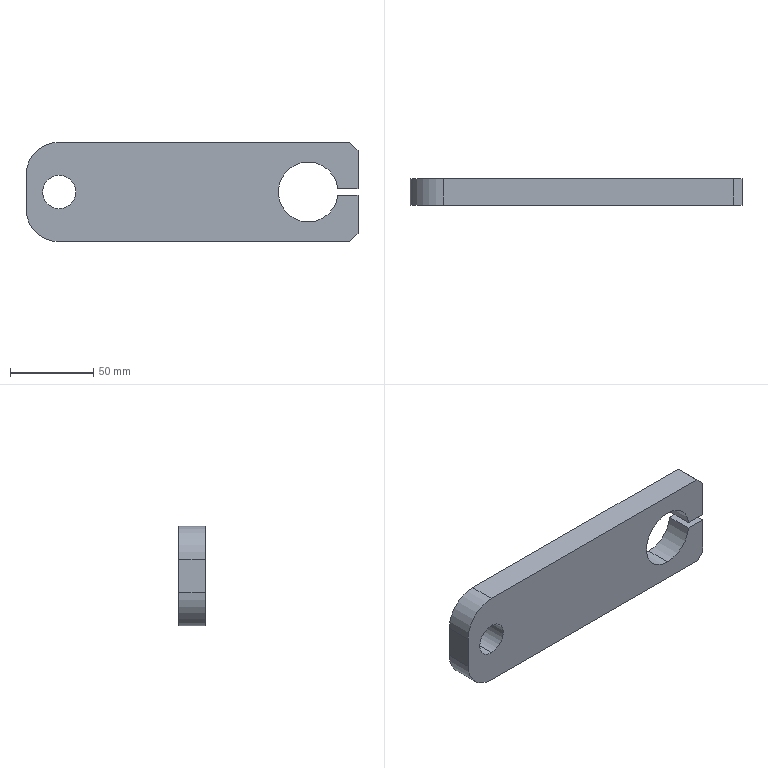Part | STEP file | PN_0015 Guide block | 1 solid | 18 faces | box 200 x 16 x 60 mm | volume 166770 mm3 | plane 11 | cylinder 7 | commonest cylinder face diameters 36 x3 20 x2 40 x2
STEP:
#1=CARTESIAN_POINT('',(0.,0.,0.));
#2=DIRECTION('',(0.,0.,1.));
#3=DIRECTION('',(1.,0.,0.));
#4=AXIS2_PLACEMENT_3D('',#1,#2,#3);
#5=CARTESIAN_POINT('',(-80.,16.,-10.));
#6=VERTEX_POINT('',#5);
#7=CARTESIAN_POINT('',(-80.,0.,-10.));
#8=VERTEX_POINT('',#7);
#9=CARTESIAN_POINT('',(-80.,16.,-10.));
#10=DIRECTION('',(0.,-1.,0.));
#11=VECTOR('',#10,1.);
#12=LINE('',#9,#11);
#13=CARTESIAN_POINT('',(-80.,16.,0.));
#14=DIRECTION('',(0.,-1.,0.));
#15=DIRECTION('',(0.,0.,-1.));
#16=AXIS2_PLACEMENT_3D('',#13,#14,#15);
#17=CYLINDRICAL_SURFACE('',#16,10.);
#18=CARTESIAN_POINT('',(6.283,0.));
#19=DIRECTION('',(0.,1.));
#20=VECTOR('',#19,1.);
#21=LINE('',#18,#20);
#22=(GEOMETRIC_REPRESENTATION_CONTEXT(2)PARAMETRIC_REPRESENTATION_CONTEXT()REPRESENTATION_CONTEXT('',''));
#23=DEFINITIONAL_REPRESENTATION('',(#21),#22);
#24=PCURVE('',#17,#23);
#25=CARTESIAN_POINT('',(-80.,16.,0.));
#26=DIRECTION('',(0.,-1.,0.));
#27=DIRECTION('',(0.,0.,-1.));
#28=AXIS2_PLACEMENT_3D('',#25,#26,#27);
#29=CYLINDRICAL_SURFACE('',#28,10.);
#30=CARTESIAN_POINT('',(0.,0.));
#31=DIRECTION('',(0.,1.));
#32=VECTOR('',#31,1.);
#33=LINE('',#30,#32);
#34=(GEOMETRIC_REPRESENTATION_CONTEXT(2)PARAMETRIC_REPRESENTATION_CONTEXT()REPRESENTATION_CONTEXT('',''));
#35=DEFINITIONAL_REPRESENTATION('',(#33),#34);
#36=PCURVE('',#29,#35);
#37=SURFACE_CURVE('',#12,(#24,#36),.PCURVE_S1.);
#38=EDGE_CURVE('',#6,#8,#37,.T.);
#39=ORIENTED_EDGE('',*,*,#38,.T.);
#40=CARTESIAN_POINT('',(-80.,0.,10.));
#41=VERTEX_POINT('',#40);
#42=CARTESIAN_POINT('',(-80.,0.,0.));
#43=DIRECTION('',(0.,1.,0.));
#44=DIRECTION('',(0.,0.,1.));
#45=AXIS2_PLACEMENT_3D('',#42,#43,#44);
#46=CIRCLE('',#45,10.);
#47=CARTESIAN_POINT('',(9.425,16.));
#48=DIRECTION('',(-1.,0.));
#49=VECTOR('',#48,1.);
#50=LINE('',#47,#49);
#51=(GEOMETRIC_REPRESENTATION_CONTEXT(2)PARAMETRIC_REPRESENTATION_CONTEXT()REPRESENTATION_CONTEXT('',''));
#52=DEFINITIONAL_REPRESENTATION('',(#50),#51);
#53=PCURVE('',#17,#52);
#54=CARTESIAN_POINT('',(70.,0.,0.));
#55=DIRECTION('',(0.,1.,0.));
#56=DIRECTION('',(0.,0.,1.));
#57=AXIS2_PLACEMENT_3D('',#54,#55,#56);
#58=PLANE('',#57);
#59=CARTESIAN_POINT('',(0.,-150.));
#60=DIRECTION('',(1.,0.));
#61=AXIS2_PLACEMENT_2D('',#59,#60);
#62=CIRCLE('',#61,10.);
#63=(GEOMETRIC_REPRESENTATION_CONTEXT(2)PARAMETRIC_REPRESENTATION_CONTEXT()REPRESENTATION_CONTEXT('',''));
#64=DEFINITIONAL_REPRESENTATION('',(#62),#63);
#65=PCURVE('',#58,#64);
#66=SURFACE_CURVE('',#46,(#53,#65),.PCURVE_S1.);
#67=EDGE_CURVE('',#8,#41,#66,.T.);
#68=ORIENTED_EDGE('',*,*,#67,.T.);
#69=CARTESIAN_POINT('',(-80.,16.,10.));
#70=VERTEX_POINT('',#69);
#71=CARTESIAN_POINT('',(-80.,16.,10.));
#72=DIRECTION('',(0.,-1.,0.));
#73=VECTOR('',#72,1.);
#74=LINE('',#71,#73);
#75=CARTESIAN_POINT('',(3.142,0.));
#76=DIRECTION('',(0.,1.));
#77=VECTOR('',#76,1.);
#78=LINE('',#75,#77);
#79=(GEOMETRIC_REPRESENTATION_CONTEXT(2)PARAMETRIC_REPRESENTATION_CONTEXT()REPRESENTATION_CONTEXT('',''));
#80=DEFINITIONAL_REPRESENTATION('',(#78),#79);
#81=PCURVE('',#17,#80);
#82=CARTESIAN_POINT('',(3.142,0.));
#83=DIRECTION('',(0.,1.));
#84=VECTOR('',#83,1.);
#85=LINE('',#82,#84);
#86=(GEOMETRIC_REPRESENTATION_CONTEXT(2)PARAMETRIC_REPRESENTATION_CONTEXT()REPRESENTATION_CONTEXT('',''));
#87=DEFINITIONAL_REPRESENTATION('',(#85),#86);
#88=PCURVE('',#29,#87);
#89=SURFACE_CURVE('',#74,(#81,#88),.PCURVE_S1.);
#90=EDGE_CURVE('',#70,#41,#89,.T.);
#91=ORIENTED_EDGE('',*,*,#90,.F.);
#92=CARTESIAN_POINT('',(-80.,16.,0.));
#93=DIRECTION('',(0.,1.,0.));
#94=DIRECTION('',(0.,0.,1.));
#95=AXIS2_PLACEMENT_3D('',#92,#93,#94);
#96=CIRCLE('',#95,10.);
#97=CARTESIAN_POINT('',(9.425,0.));
#98=DIRECTION('',(-1.,0.));
#99=VECTOR('',#98,1.);
#100=LINE('',#97,#99);
#101=(GEOMETRIC_REPRESENTATION_CONTEXT(2)PARAMETRIC_REPRESENTATION_CONTEXT()REPRESENTATION_CONTEXT('',''));
#102=DEFINITIONAL_REPRESENTATION('',(#100),#101);
#103=PCURVE('',#17,#102);
#104=CARTESIAN_POINT('',(70.,16.,0.));
#105=DIRECTION('',(0.,1.,0.));
#106=DIRECTION('',(0.,0.,1.));
#107=AXIS2_PLACEMENT_3D('',#104,#105,#106);
#108=PLANE('',#107);
#109=CARTESIAN_POINT('',(0.,-150.));
#110=DIRECTION('',(1.,0.));
#111=AXIS2_PLACEMENT_2D('',#109,#110);
#112=CIRCLE('',#111,10.);
#113=(GEOMETRIC_REPRESENTATION_CONTEXT(2)PARAMETRIC_REPRESENTATION_CONTEXT()REPRESENTATION_CONTEXT('',''));
#114=DEFINITIONAL_REPRESENTATION('',(#112),#113);
#115=PCURVE('',#108,#114);
#116=SURFACE_CURVE('',#96,(#103,#115),.PCURVE_S1.);
#117=EDGE_CURVE('',#6,#70,#116,.T.);
#118=ORIENTED_EDGE('',*,*,#117,.F.);
#119=EDGE_LOOP('',(#39,#68,#91,#118));
#120=FACE_BOUND('',#119,.F.);
#121=ADVANCED_FACE('',(#120),#17,.F.);
#122=CARTESIAN_POINT('',(70.,16.,-18.));
#123=VERTEX_POINT('',#122);
#124=CARTESIAN_POINT('',(70.,0.,-18.));
#125=VERTEX_POINT('',#124);
#126=CARTESIAN_POINT('',(70.,16.,-18.));
#127=DIRECTION('',(0.,-1.,0.));
#128=VECTOR('',#127,1.);
#129=LINE('',#126,#128);
#130=CARTESIAN_POINT('',(70.,16.,0.));
#131=DIRECTION('',(0.,-1.,0.));
#132=DIRECTION('',(0.,0.,-1.));
#133=AXIS2_PLACEMENT_3D('',#130,#131,#132);
#134=CYLINDRICAL_SURFACE('',#133,18.);
#135=CARTESIAN_POINT('',(6.283,0.));
#136=DIRECTION('',(0.,1.));
#137=VECTOR('',#136,1.);
#138=LINE('',#135,#137);
#139=(GEOMETRIC_REPRESENTATION_CONTEXT(2)PARAMETRIC_REPRESENTATION_CONTEXT()REPRESENTATION_CONTEXT('',''));
#140=DEFINITIONAL_REPRESENTATION('',(#138),#139);
#141=PCURVE('',#134,#140);
#142=CARTESIAN_POINT('',(70.,16.,0.));
#143=DIRECTION('',(0.,-1.,0.));
#144=DIRECTION('',(0.,0.,-1.));
#145=AXIS2_PLACEMENT_3D('',#142,#143,#144);
#146=CYLINDRICAL_SURFACE('',#145,18.);
#147=CARTESIAN_POINT('',(0.,0.));
#148=DIRECTION('',(0.,1.));
#149=VECTOR('',#148,1.);
#150=LINE('',#147,#149);
#151=(GEOMETRIC_REPRESENTATION_CONTEXT(2)PARAMETRIC_REPRESENTATION_CONTEXT()REPRESENTATION_CONTEXT('',''));
#152=DEFINITIONAL_REPRESENTATION('',(#150),#151);
#153=PCURVE('',#146,#152);
#154=SURFACE_CURVE('',#129,(#141,#153),.PCURVE_S1.);
#155=EDGE_CURVE('',#123,#125,#154,.T.);
#156=ORIENTED_EDGE('',*,*,#155,.T.);
#157=CARTESIAN_POINT('',(70.,0.,18.));
#158=VERTEX_POINT('',#157);
#159=CARTESIAN_POINT('',(70.,0.,0.));
#160=DIRECTION('',(0.,-1.,0.));
#161=DIRECTION('',(0.,0.,1.));
#162=AXIS2_PLACEMENT_3D('',#159,#160,#161);
#163=CIRCLE('',#162,18.);
#164=CARTESIAN_POINT('',(3.142,16.));
#165=DIRECTION('',(1.,0.));
#166=VECTOR('',#165,1.);
#167=LINE('',#164,#166);
#168=(GEOMETRIC_REPRESENTATION_CONTEXT(2)PARAMETRIC_REPRESENTATION_CONTEXT()REPRESENTATION_CONTEXT('',''));
#169=DEFINITIONAL_REPRESENTATION('',(#167),#168);
#170=PCURVE('',#134,#169);
#171=CARTESIAN_POINT('',(18.,0.));
#172=CARTESIAN_POINT('',(18.,-31.177));
#173=CARTESIAN_POINT('',(-9.,-15.588));
#174=CARTESIAN_POINT('',(-36.,0.));
#175=CARTESIAN_POINT('',(-9.,15.588));
#176=CARTESIAN_POINT('',(18.,31.177));
#177=CARTESIAN_POINT('',(18.,0.));
#178=(BOUNDED_CURVE()B_SPLINE_CURVE(2,(#171,#172,#173,#174,#175,#176,#177),.UNSPECIFIED.,.T.,.F.)B_SPLINE_CURVE_WITH_KNOTS((1,2,2,2,2,1),(-2.094,0.,2.094,4.189,6.283,8.378),.UNSPECIFIED.)CURVE()GEOMETRIC_REPRESENTATION_ITEM()RATIONAL_B_SPLINE_CURVE((1.,0.5,1.,0.5,1.,0.5,1.))REPRESENTATION_ITEM(''));
#179=(GEOMETRIC_REPRESENTATION_CONTEXT(2)PARAMETRIC_REPRESENTATION_CONTEXT()REPRESENTATION_CONTEXT('',''));
#180=DEFINITIONAL_REPRESENTATION('',(#178),#179);
#181=PCURVE('',#58,#180);
#182=SURFACE_CURVE('',#163,(#170,#181),.PCURVE_S1.);
#183=EDGE_CURVE('',#158,#125,#182,.T.);
#184=ORIENTED_EDGE('',*,*,#183,.F.);
#185=CARTESIAN_POINT('',(70.,16.,18.));
#186=VERTEX_POINT('',#185);
#187=CARTESIAN_POINT('',(70.,16.,18.));
#188=DIRECTION('',(0.,-1.,0.));
#189=VECTOR('',#188,1.);
#190=LINE('',#187,#189);
#191=CARTESIAN_POINT('',(3.142,0.));
#192=DIRECTION('',(0.,1.));
#193=VECTOR('',#192,1.);
#194=LINE('',#191,#193);
#195=(GEOMETRIC_REPRESENTATION_CONTEXT(2)PARAMETRIC_REPRESENTATION_CONTEXT()REPRESENTATION_CONTEXT('',''));
#196=DEFINITIONAL_REPRESENTATION('',(#194),#195);
#197=PCURVE('',#134,#196);
#198=CARTESIAN_POINT('',(70.,16.,0.));
#199=DIRECTION('',(0.,-1.,0.));
#200=DIRECTION('',(0.,0.,-1.));
#201=AXIS2_PLACEMENT_3D('',#198,#199,#200);
#202=CYLINDRICAL_SURFACE('',#201,18.);
#203=CARTESIAN_POINT('',(3.142,0.));
#204=DIRECTION('',(0.,1.));
#205=VECTOR('',#204,1.);
#206=LINE('',#203,#205);
#207=(GEOMETRIC_REPRESENTATION_CONTEXT(2)PARAMETRIC_REPRESENTATION_CONTEXT()REPRESENTATION_CONTEXT('',''));
#208=DEFINITIONAL_REPRESENTATION('',(#206),#207);
#209=PCURVE('',#202,#208);
#210=SURFACE_CURVE('',#190,(#197,#209),.PCURVE_S1.);
#211=EDGE_CURVE('',#186,#158,#210,.T.);
#212=ORIENTED_EDGE('',*,*,#211,.F.);
#213=CARTESIAN_POINT('',(70.,16.,0.));
#214=DIRECTION('',(0.,-1.,0.));
#215=DIRECTION('',(0.,0.,1.));
#216=AXIS2_PLACEMENT_3D('',#213,#214,#215);
#217=CIRCLE('',#216,18.);
#218=CARTESIAN_POINT('',(3.142,0.));
#219=DIRECTION('',(1.,0.));
#220=VECTOR('',#219,1.);
#221=LINE('',#218,#220);
#222=(GEOMETRIC_REPRESENTATION_CONTEXT(2)PARAMETRIC_REPRESENTATION_CONTEXT()REPRESENTATION_CONTEXT('',''));
#223=DEFINITIONAL_REPRESENTATION('',(#221),#222);
#224=PCURVE('',#134,#223);
#225=CARTESIAN_POINT('',(18.,0.));
#226=CARTESIAN_POINT('',(18.,-31.177));
#227=CARTESIAN_POINT('',(-9.,-15.588));
#228=CARTESIAN_POINT('',(-36.,0.));
#229=CARTESIAN_POINT('',(-9.,15.588));
#230=CARTESIAN_POINT('',(18.,31.177));
#231=CARTESIAN_POINT('',(18.,0.));
#232=(BOUNDED_CURVE()B_SPLINE_CURVE(2,(#225,#226,#227,#228,#229,#230,#231),.UNSPECIFIED.,.T.,.F.)B_SPLINE_CURVE_WITH_KNOTS((1,2,2,2,2,1),(-2.094,0.,2.094,4.189,6.283,8.378),.UNSPECIFIED.)CURVE()GEOMETRIC_REPRESENTATION_ITEM()RATIONAL_B_SPLINE_CURVE((1.,0.5,1.,0.5,1.,0.5,1.))REPRESENTATION_ITEM(''));
#233=(GEOMETRIC_REPRESENTATION_CONTEXT(2)PARAMETRIC_REPRESENTATION_CONTEXT()REPRESENTATION_CONTEXT('',''));
#234=DEFINITIONAL_REPRESENTATION('',(#232),#233);
#235=PCURVE('',#108,#234);
#236=SURFACE_CURVE('',#217,(#224,#235),.PCURVE_S1.);
#237=EDGE_CURVE('',#186,#123,#236,.T.);
#238=ORIENTED_EDGE('',*,*,#237,.T.);
#239=EDGE_LOOP('',(#156,#184,#212,#238));
#240=FACE_BOUND('',#239,.F.);
#241=ADVANCED_FACE('',(#240),#134,.F.);
#242=CARTESIAN_POINT('',(87.889,16.,-2.));
#243=VERTEX_POINT('',#242);
#244=CARTESIAN_POINT('',(87.889,0.,-2.));
#245=VERTEX_POINT('',#244);
#246=CARTESIAN_POINT('',(87.889,16.,-2.));
#247=DIRECTION('',(0.,-1.,0.));
#248=VECTOR('',#247,1.);
#249=LINE('',#246,#248);
#250=CARTESIAN_POINT('',(1.459,0.));
#251=DIRECTION('',(0.,1.));
#252=VECTOR('',#251,1.);
#253=LINE('',#250,#252);
#254=(GEOMETRIC_REPRESENTATION_CONTEXT(2)PARAMETRIC_REPRESENTATION_CONTEXT()REPRESENTATION_CONTEXT('',''));
#255=DEFINITIONAL_REPRESENTATION('',(#253),#254);
#256=PCURVE('',#146,#255);
#257=CARTESIAN_POINT('',(87.889,16.,-2.));
#258=DIRECTION('',(0.,0.,-1.));
#259=DIRECTION('',(-1.,0.,0.));
#260=AXIS2_PLACEMENT_3D('',#257,#258,#259);
#261=PLANE('',#260);
#262=CARTESIAN_POINT('',(0.,0.));
#263=DIRECTION('',(0.,-1.));
#264=VECTOR('',#263,1.);
#265=LINE('',#262,#264);
#266=(GEOMETRIC_REPRESENTATION_CONTEXT(2)PARAMETRIC_REPRESENTATION_CONTEXT()REPRESENTATION_CONTEXT('',''));
#267=DEFINITIONAL_REPRESENTATION('',(#265),#266);
#268=PCURVE('',#261,#267);
#269=SURFACE_CURVE('',#249,(#256,#268),.PCURVE_S1.);
#270=EDGE_CURVE('',#243,#245,#269,.T.);
#271=ORIENTED_EDGE('',*,*,#270,.T.);
#272=CARTESIAN_POINT('',(70.,0.,0.));
#273=DIRECTION('',(0.,-1.,0.));
#274=DIRECTION('',(0.,0.,1.));
#275=AXIS2_PLACEMENT_3D('',#272,#273,#274);
#276=CIRCLE('',#275,18.);
#277=CARTESIAN_POINT('',(-3.142,16.));
#278=DIRECTION('',(1.,0.));
#279=VECTOR('',#278,1.);
#280=LINE('',#277,#279);
#281=(GEOMETRIC_REPRESENTATION_CONTEXT(2)PARAMETRIC_REPRESENTATION_CONTEXT()REPRESENTATION_CONTEXT('',''));
#282=DEFINITIONAL_REPRESENTATION('',(#280),#281);
#283=PCURVE('',#146,#282);
#284=CARTESIAN_POINT('',(18.,0.));
#285=CARTESIAN_POINT('',(18.,-31.177));
#286=CARTESIAN_POINT('',(-9.,-15.588));
#287=CARTESIAN_POINT('',(-36.,0.));
#288=CARTESIAN_POINT('',(-9.,15.588));
#289=CARTESIAN_POINT('',(18.,31.177));
#290=CARTESIAN_POINT('',(18.,0.));
#291=(BOUNDED_CURVE()B_SPLINE_CURVE(2,(#284,#285,#286,#287,#288,#289,#290),.UNSPECIFIED.,.T.,.F.)B_SPLINE_CURVE_WITH_KNOTS((1,2,2,2,2,1),(-2.094,0.,2.094,4.189,6.283,8.378),.UNSPECIFIED.)CURVE()GEOMETRIC_REPRESENTATION_ITEM()RATIONAL_B_SPLINE_CURVE((1.,0.5,1.,0.5,1.,0.5,1.))REPRESENTATION_ITEM(''));
#292=(GEOMETRIC_REPRESENTATION_CONTEXT(2)PARAMETRIC_REPRESENTATION_CONTEXT()REPRESENTATION_CONTEXT('',''));
#293=DEFINITIONAL_REPRESENTATION('',(#291),#292);
#294=PCURVE('',#58,#293);
#295=SURFACE_CURVE('',#276,(#283,#294),.PCURVE_S1.);
#296=EDGE_CURVE('',#125,#245,#295,.T.);
#297=ORIENTED_EDGE('',*,*,#296,.F.);
#298=ORIENTED_EDGE('',*,*,#155,.F.);
#299=CARTESIAN_POINT('',(70.,16.,0.));
#300=DIRECTION('',(0.,-1.,0.));
#301=DIRECTION('',(0.,0.,1.));
#302=AXIS2_PLACEMENT_3D('',#299,#300,#301);
#303=CIRCLE('',#302,18.);
#304=CARTESIAN_POINT('',(-3.142,0.));
#305=DIRECTION('',(1.,0.));
#306=VECTOR('',#305,1.);
#307=LINE('',#304,#306);
#308=(GEOMETRIC_REPRESENTATION_CONTEXT(2)PARAMETRIC_REPRESENTATION_CONTEXT()REPRESENTATION_CONTEXT('',''));
#309=DEFINITIONAL_REPRESENTATION('',(#307),#308);
#310=PCURVE('',#146,#309);
#311=CARTESIAN_POINT('',(18.,0.));
#312=CARTESIAN_POINT('',(18.,-31.177));
#313=CARTESIAN_POINT('',(-9.,-15.588));
#314=CARTESIAN_POINT('',(-36.,0.));
#315=CARTESIAN_POINT('',(-9.,15.588));
#316=CARTESIAN_POINT('',(18.,31.177));
#317=CARTESIAN_POINT('',(18.,0.));
#318=(BOUNDED_CURVE()B_SPLINE_CURVE(2,(#311,#312,#313,#314,#315,#316,#317),.UNSPECIFIED.,.T.,.F.)B_SPLINE_CURVE_WITH_KNOTS((1,2,2,2,2,1),(-2.094,0.,2.094,4.189,6.283,8.378),.UNSPECIFIED.)CURVE()GEOMETRIC_REPRESENTATION_ITEM()RATIONAL_B_SPLINE_CURVE((1.,0.5,1.,0.5,1.,0.5,1.))REPRESENTATION_ITEM(''));
#319=(GEOMETRIC_REPRESENTATION_CONTEXT(2)PARAMETRIC_REPRESENTATION_CONTEXT()REPRESENTATION_CONTEXT('',''));
#320=DEFINITIONAL_REPRESENTATION('',(#318),#319);
#321=PCURVE('',#108,#320);
#322=SURFACE_CURVE('',#303,(#310,#321),.PCURVE_S1.);
#323=EDGE_CURVE('',#123,#243,#322,.T.);
#324=ORIENTED_EDGE('',*,*,#323,.T.);
#325=EDGE_LOOP('',(#271,#297,#298,#324));
#326=FACE_BOUND('',#325,.F.);
#327=ADVANCED_FACE('',(#326),#146,.F.);
#328=CARTESIAN_POINT('',(-80.,16.,30.));
#329=VERTEX_POINT('',#328);
#330=CARTESIAN_POINT('',(95.,16.,30.));
#331=VERTEX_POINT('',#330);
#332=CARTESIAN_POINT('',(-100.,16.,30.));
#333=DIRECTION('',(1.,0.,0.));
#334=VECTOR('',#333,1.);
#335=LINE('',#332,#334);
#336=CARTESIAN_POINT('',(30.,-170.));
#337=DIRECTION('',(0.,1.));
#338=VECTOR('',#337,1.);
#339=LINE('',#336,#338);
#340=(GEOMETRIC_REPRESENTATION_CONTEXT(2)PARAMETRIC_REPRESENTATION_CONTEXT()REPRESENTATION_CONTEXT('',''));
#341=DEFINITIONAL_REPRESENTATION('',(#339),#340);
#342=PCURVE('',#108,#341);
#343=CARTESIAN_POINT('',(-100.,16.,30.));
#344=DIRECTION('',(0.,0.,-1.));
#345=DIRECTION('',(-1.,0.,0.));
#346=AXIS2_PLACEMENT_3D('',#343,#344,#345);
#347=PLANE('',#346);
#348=CARTESIAN_POINT('',(0.,0.));
#349=DIRECTION('',(-1.,0.));
#350=VECTOR('',#349,1.);
#351=LINE('',#348,#350);
#352=(GEOMETRIC_REPRESENTATION_CONTEXT(2)PARAMETRIC_REPRESENTATION_CONTEXT()REPRESENTATION_CONTEXT('',''));
#353=DEFINITIONAL_REPRESENTATION('',(#351),#352);
#354=PCURVE('',#347,#353);
#355=SURFACE_CURVE('',#335,(#342,#354),.PCURVE_S1.);
#356=EDGE_CURVE('',#329,#331,#355,.T.);
#357=ORIENTED_EDGE('',*,*,#356,.T.);
#358=CARTESIAN_POINT('',(100.,16.,25.));
#359=VERTEX_POINT('',#358);
#360=CARTESIAN_POINT('',(97.5,16.,27.5));
#361=DIRECTION('',(0.7071,0.,-0.7071));
#362=VECTOR('',#361,1.);
#363=LINE('',#360,#362);
#364=CARTESIAN_POINT('',(27.5,27.5));
#365=DIRECTION('',(-0.7071,0.7071));
#366=VECTOR('',#365,1.);
#367=LINE('',#364,#366);
#368=(GEOMETRIC_REPRESENTATION_CONTEXT(2)PARAMETRIC_REPRESENTATION_CONTEXT()REPRESENTATION_CONTEXT('',''));
#369=DEFINITIONAL_REPRESENTATION('',(#367),#368);
#370=PCURVE('',#108,#369);
#371=CARTESIAN_POINT('',(100.,16.,25.));
#372=DIRECTION('',(-0.7071,0.,-0.7071));
#373=DIRECTION('',(-0.7071,0.,0.7071));
#374=AXIS2_PLACEMENT_3D('',#371,#372,#373);
#375=PLANE('',#374);
#376=CARTESIAN_POINT('',(3.536,0.));
#377=DIRECTION('',(-1.,0.));
#378=VECTOR('',#377,1.);
#379=LINE('',#376,#378);
#380=(GEOMETRIC_REPRESENTATION_CONTEXT(2)PARAMETRIC_REPRESENTATION_CONTEXT()REPRESENTATION_CONTEXT('',''));
#381=DEFINITIONAL_REPRESENTATION('',(#379),#380);
#382=PCURVE('',#375,#381);
#383=SURFACE_CURVE('',#363,(#370,#382),.PCURVE_S1.);
#384=EDGE_CURVE('',#331,#359,#383,.T.);
#385=ORIENTED_EDGE('',*,*,#384,.T.);
#386=CARTESIAN_POINT('',(100.,16.,2.));
#387=VERTEX_POINT('',#386);
#388=CARTESIAN_POINT('',(100.,16.,2.));
#389=DIRECTION('',(0.,0.,-1.));
#390=VECTOR('',#389,1.);
#391=LINE('',#388,#390);
#392=CARTESIAN_POINT('',(2.,30.));
#393=DIRECTION('',(-1.,0.));
#394=VECTOR('',#393,1.);
#395=LINE('',#392,#394);
#396=(GEOMETRIC_REPRESENTATION_CONTEXT(2)PARAMETRIC_REPRESENTATION_CONTEXT()REPRESENTATION_CONTEXT('',''));
#397=DEFINITIONAL_REPRESENTATION('',(#395),#396);
#398=PCURVE('',#108,#397);
#399=CARTESIAN_POINT('',(100.,16.,2.));
#400=DIRECTION('',(-1.,0.,0.));
#401=DIRECTION('',(0.,0.,1.));
#402=AXIS2_PLACEMENT_3D('',#399,#400,#401);
#403=PLANE('',#402);
#404=CARTESIAN_POINT('',(0.,0.));
#405=DIRECTION('',(-1.,0.));
#406=VECTOR('',#405,1.);
#407=LINE('',#404,#406);
#408=(GEOMETRIC_REPRESENTATION_CONTEXT(2)PARAMETRIC_REPRESENTATION_CONTEXT()REPRESENTATION_CONTEXT('',''));
#409=DEFINITIONAL_REPRESENTATION('',(#407),#408);
#410=PCURVE('',#403,#409);
#411=SURFACE_CURVE('',#391,(#398,#410),.PCURVE_S1.);
#412=EDGE_CURVE('',#359,#387,#411,.T.);
#413=ORIENTED_EDGE('',*,*,#412,.T.);
#414=CARTESIAN_POINT('',(87.889,16.,2.));
#415=VERTEX_POINT('',#414);
#416=CARTESIAN_POINT('',(87.889,16.,2.));
#417=DIRECTION('',(-1.,0.,0.));
#418=VECTOR('',#417,1.);
#419=LINE('',#416,#418);
#420=CARTESIAN_POINT('',(2.,17.889));
#421=DIRECTION('',(0.,-1.));
#422=VECTOR('',#421,1.);
#423=LINE('',#420,#422);
#424=(GEOMETRIC_REPRESENTATION_CONTEXT(2)PARAMETRIC_REPRESENTATION_CONTEXT()REPRESENTATION_CONTEXT('',''));
#425=DEFINITIONAL_REPRESENTATION('',(#423),#424);
#426=PCURVE('',#108,#425);
#427=CARTESIAN_POINT('',(87.889,16.,2.));
#428=DIRECTION('',(0.,0.,1.));
#429=DIRECTION('',(1.,0.,0.));
#430=AXIS2_PLACEMENT_3D('',#427,#428,#429);
#431=PLANE('',#430);
#432=CARTESIAN_POINT('',(0.,0.));
#433=DIRECTION('',(-1.,0.));
#434=VECTOR('',#433,1.);
#435=LINE('',#432,#434);
#436=(GEOMETRIC_REPRESENTATION_CONTEXT(2)PARAMETRIC_REPRESENTATION_CONTEXT()REPRESENTATION_CONTEXT('',''));
#437=DEFINITIONAL_REPRESENTATION('',(#435),#436);
#438=PCURVE('',#431,#437);
#439=SURFACE_CURVE('',#419,(#426,#438),.PCURVE_S1.);
#440=EDGE_CURVE('',#387,#415,#439,.T.);
#441=ORIENTED_EDGE('',*,*,#440,.T.);
#442=CARTESIAN_POINT('',(70.,16.,0.));
#443=DIRECTION('',(0.,-1.,0.));
#444=DIRECTION('',(0.,0.,1.));
#445=AXIS2_PLACEMENT_3D('',#442,#443,#444);
#446=CIRCLE('',#445,18.);
#447=CARTESIAN_POINT('',(18.,0.));
#448=CARTESIAN_POINT('',(18.,-31.177));
#449=CARTESIAN_POINT('',(-9.,-15.588));
#450=CARTESIAN_POINT('',(-36.,0.));
#451=CARTESIAN_POINT('',(-9.,15.588));
#452=CARTESIAN_POINT('',(18.,31.177));
#453=CARTESIAN_POINT('',(18.,0.));
#454=(BOUNDED_CURVE()B_SPLINE_CURVE(2,(#447,#448,#449,#450,#451,#452,#453),.UNSPECIFIED.,.T.,.F.)B_SPLINE_CURVE_WITH_KNOTS((1,2,2,2,2,1),(-2.094,0.,2.094,4.189,6.283,8.378),.UNSPECIFIED.)CURVE()GEOMETRIC_REPRESENTATION_ITEM()RATIONAL_B_SPLINE_CURVE((1.,0.5,1.,0.5,1.,0.5,1.))REPRESENTATION_ITEM(''));
#455=(GEOMETRIC_REPRESENTATION_CONTEXT(2)PARAMETRIC_REPRESENTATION_CONTEXT()REPRESENTATION_CONTEXT('',''));
#456=DEFINITIONAL_REPRESENTATION('',(#454),#455);
#457=PCURVE('',#108,#456);
#458=CARTESIAN_POINT('',(-3.142,0.));
#459=DIRECTION('',(1.,0.));
#460=VECTOR('',#459,1.);
#461=LINE('',#458,#460);
#462=(GEOMETRIC_REPRESENTATION_CONTEXT(2)PARAMETRIC_REPRESENTATION_CONTEXT()REPRESENTATION_CONTEXT('',''));
#463=DEFINITIONAL_REPRESENTATION('',(#461),#462);
#464=PCURVE('',#202,#463);
#465=SURFACE_CURVE('',#446,(#457,#464),.PCURVE_S1.);
#466=EDGE_CURVE('',#415,#186,#465,.T.);
#467=ORIENTED_EDGE('',*,*,#466,.T.);
#468=ORIENTED_EDGE('',*,*,#237,.T.);
#469=ORIENTED_EDGE('',*,*,#323,.T.);
#470=CARTESIAN_POINT('',(100.,16.,-2.));
#471=VERTEX_POINT('',#470);
#472=CARTESIAN_POINT('',(87.889,16.,-2.));
#473=DIRECTION('',(1.,0.,0.));
#474=VECTOR('',#473,1.);
#475=LINE('',#472,#474);
#476=CARTESIAN_POINT('',(-2.,17.889));
#477=DIRECTION('',(0.,1.));
#478=VECTOR('',#477,1.);
#479=LINE('',#476,#478);
#480=(GEOMETRIC_REPRESENTATION_CONTEXT(2)PARAMETRIC_REPRESENTATION_CONTEXT()REPRESENTATION_CONTEXT('',''));
#481=DEFINITIONAL_REPRESENTATION('',(#479),#480);
#482=PCURVE('',#108,#481);
#483=CARTESIAN_POINT('',(0.,0.));
#484=DIRECTION('',(-1.,0.));
#485=VECTOR('',#484,1.);
#486=LINE('',#483,#485);
#487=(GEOMETRIC_REPRESENTATION_CONTEXT(2)PARAMETRIC_REPRESENTATION_CONTEXT()REPRESENTATION_CONTEXT('',''));
#488=DEFINITIONAL_REPRESENTATION('',(#486),#487);
#489=PCURVE('',#261,#488);
#490=SURFACE_CURVE('',#475,(#482,#489),.PCURVE_S1.);
#491=EDGE_CURVE('',#243,#471,#490,.T.);
#492=ORIENTED_EDGE('',*,*,#491,.T.);
#493=CARTESIAN_POINT('',(100.,16.,-25.));
#494=VERTEX_POINT('',#493);
#495=CARTESIAN_POINT('',(100.,16.,-30.));
#496=DIRECTION('',(0.,0.,-1.));
#497=VECTOR('',#496,1.);
#498=LINE('',#495,#497);
#499=CARTESIAN_POINT('',(-30.,30.));
#500=DIRECTION('',(-1.,0.));
#501=VECTOR('',#500,1.);
#502=LINE('',#499,#501);
#503=(GEOMETRIC_REPRESENTATION_CONTEXT(2)PARAMETRIC_REPRESENTATION_CONTEXT()REPRESENTATION_CONTEXT('',''));
#504=DEFINITIONAL_REPRESENTATION('',(#502),#503);
#505=PCURVE('',#108,#504);
#506=CARTESIAN_POINT('',(100.,16.,-30.));
#507=DIRECTION('',(-1.,0.,0.));
#508=DIRECTION('',(0.,0.,1.));
#509=AXIS2_PLACEMENT_3D('',#506,#507,#508);
#510=PLANE('',#509);
#511=CARTESIAN_POINT('',(0.,0.));
#512=DIRECTION('',(-1.,0.));
#513=VECTOR('',#512,1.);
#514=LINE('',#511,#513);
#515=(GEOMETRIC_REPRESENTATION_CONTEXT(2)PARAMETRIC_REPRESENTATION_CONTEXT()REPRESENTATION_CONTEXT('',''));
#516=DEFINITIONAL_REPRESENTATION('',(#514),#515);
#517=PCURVE('',#510,#516);
#518=SURFACE_CURVE('',#498,(#505,#517),.PCURVE_S1.);
#519=EDGE_CURVE('',#471,#494,#518,.T.);
#520=ORIENTED_EDGE('',*,*,#519,.T.);
#521=CARTESIAN_POINT('',(95.,16.,-30.));
#522=VERTEX_POINT('',#521);
#523=CARTESIAN_POINT('',(97.5,16.,-27.5));
#524=DIRECTION('',(-0.7071,0.,-0.7071));
#525=VECTOR('',#524,1.);
#526=LINE('',#523,#525);
#527=CARTESIAN_POINT('',(-27.5,27.5));
#528=DIRECTION('',(-0.7071,-0.7071));
#529=VECTOR('',#528,1.);
#530=LINE('',#527,#529);
#531=(GEOMETRIC_REPRESENTATION_CONTEXT(2)PARAMETRIC_REPRESENTATION_CONTEXT()REPRESENTATION_CONTEXT('',''));
#532=DEFINITIONAL_REPRESENTATION('',(#530),#531);
#533=PCURVE('',#108,#532);
#534=CARTESIAN_POINT('',(95.,16.,-30.));
#535=DIRECTION('',(-0.7071,0.,0.7071));
#536=DIRECTION('',(0.7071,0.,0.7071));
#537=AXIS2_PLACEMENT_3D('',#534,#535,#536);
#538=PLANE('',#537);
#539=CARTESIAN_POINT('',(3.536,0.));
#540=DIRECTION('',(-1.,0.));
#541=VECTOR('',#540,1.);
#542=LINE('',#539,#541);
#543=(GEOMETRIC_REPRESENTATION_CONTEXT(2)PARAMETRIC_REPRESENTATION_CONTEXT()REPRESENTATION_CONTEXT('',''));
#544=DEFINITIONAL_REPRESENTATION('',(#542),#543);
#545=PCURVE('',#538,#544);
#546=SURFACE_CURVE('',#526,(#533,#545),.PCURVE_S1.);
#547=EDGE_CURVE('',#494,#522,#546,.T.);
#548=ORIENTED_EDGE('',*,*,#547,.T.);
#549=CARTESIAN_POINT('',(-80.,16.,-30.));
#550=VERTEX_POINT('',#549);
#551=CARTESIAN_POINT('',(-100.,16.,-30.));
#552=DIRECTION('',(-1.,0.,0.));
#553=VECTOR('',#552,1.);
#554=LINE('',#551,#553);
#555=CARTESIAN_POINT('',(-30.,-170.));
#556=DIRECTION('',(0.,-1.));
#557=VECTOR('',#556,1.);
#558=LINE('',#555,#557);
#559=(GEOMETRIC_REPRESENTATION_CONTEXT(2)PARAMETRIC_REPRESENTATION_CONTEXT()REPRESENTATION_CONTEXT('',''));
#560=DEFINITIONAL_REPRESENTATION('',(#558),#559);
#561=PCURVE('',#108,#560);
#562=CARTESIAN_POINT('',(-100.,16.,-30.));
#563=DIRECTION('',(0.,0.,1.));
#564=DIRECTION('',(1.,0.,0.));
#565=AXIS2_PLACEMENT_3D('',#562,#563,#564);
#566=PLANE('',#565);
#567=CARTESIAN_POINT('',(0.,0.));
#568=DIRECTION('',(-1.,0.));
#569=VECTOR('',#568,1.);
#570=LINE('',#567,#569);
#571=(GEOMETRIC_REPRESENTATION_CONTEXT(2)PARAMETRIC_REPRESENTATION_CONTEXT()REPRESENTATION_CONTEXT('',''));
#572=DEFINITIONAL_REPRESENTATION('',(#570),#571);
#573=PCURVE('',#566,#572);
#574=SURFACE_CURVE('',#554,(#561,#573),.PCURVE_S1.);
#575=EDGE_CURVE('',#522,#550,#574,.T.);
#576=ORIENTED_EDGE('',*,*,#575,.T.);
#577=CARTESIAN_POINT('',(-100.,16.,-10.));
#578=VERTEX_POINT('',#577);
#579=CARTESIAN_POINT('',(-80.,16.,-10.));
#580=DIRECTION('',(0.,1.,0.));
#581=DIRECTION('',(0.,0.,1.));
#582=AXIS2_PLACEMENT_3D('',#579,#580,#581);
#583=CIRCLE('',#582,20.);
#584=CARTESIAN_POINT('',(-10.,-150.));
#585=DIRECTION('',(1.,0.));
#586=AXIS2_PLACEMENT_2D('',#584,#585);
#587=CIRCLE('',#586,20.);
#588=(GEOMETRIC_REPRESENTATION_CONTEXT(2)PARAMETRIC_REPRESENTATION_CONTEXT()REPRESENTATION_CONTEXT('',''));
#589=DEFINITIONAL_REPRESENTATION('',(#587),#588);
#590=PCURVE('',#108,#589);
#591=CARTESIAN_POINT('',(-80.,16.,-10.));
#592=DIRECTION('',(0.,-1.,0.));
#593=DIRECTION('',(0.,0.,-1.));
#594=AXIS2_PLACEMENT_3D('',#591,#592,#593);
#595=CYLINDRICAL_SURFACE('',#594,20.);
#596=CARTESIAN_POINT('',(9.425,0.));
#597=DIRECTION('',(-1.,0.));
#598=VECTOR('',#597,1.);
#599=LINE('',#596,#598);
#600=(GEOMETRIC_REPRESENTATION_CONTEXT(2)PARAMETRIC_REPRESENTATION_CONTEXT()REPRESENTATION_CONTEXT('',''));
#601=DEFINITIONAL_REPRESENTATION('',(#599),#600);
#602=PCURVE('',#595,#601);
#603=SURFACE_CURVE('',#583,(#590,#602),.PCURVE_S1.);
#604=EDGE_CURVE('',#550,#578,#603,.T.);
#605=ORIENTED_EDGE('',*,*,#604,.T.);
#606=CARTESIAN_POINT('',(-100.,16.,10.));
#607=VERTEX_POINT('',#606);
#608=CARTESIAN_POINT('',(-100.,16.,-30.));
#609=DIRECTION('',(0.,0.,1.));
#610=VECTOR('',#609,1.);
#611=LINE('',#608,#610);
#612=CARTESIAN_POINT('',(-30.,-170.));
#613=DIRECTION('',(1.,0.));
#614=VECTOR('',#613,1.);
#615=LINE('',#612,#614);
#616=(GEOMETRIC_REPRESENTATION_CONTEXT(2)PARAMETRIC_REPRESENTATION_CONTEXT()REPRESENTATION_CONTEXT('',''));
#617=DEFINITIONAL_REPRESENTATION('',(#615),#616);
#618=PCURVE('',#108,#617);
#619=CARTESIAN_POINT('',(-100.,16.,-30.));
#620=DIRECTION('',(1.,0.,0.));
#621=DIRECTION('',(0.,0.,-1.));
#622=AXIS2_PLACEMENT_3D('',#619,#620,#621);
#623=PLANE('',#622);
#624=CARTESIAN_POINT('',(0.,0.));
#625=DIRECTION('',(-1.,0.));
#626=VECTOR('',#625,1.);
#627=LINE('',#624,#626);
#628=(GEOMETRIC_REPRESENTATION_CONTEXT(2)PARAMETRIC_REPRESENTATION_CONTEXT()REPRESENTATION_CONTEXT('',''));
#629=DEFINITIONAL_REPRESENTATION('',(#627),#628);
#630=PCURVE('',#623,#629);
#631=SURFACE_CURVE('',#611,(#618,#630),.PCURVE_S1.);
#632=EDGE_CURVE('',#578,#607,#631,.T.);
#633=ORIENTED_EDGE('',*,*,#632,.T.);
#634=CARTESIAN_POINT('',(-80.,16.,10.));
#635=DIRECTION('',(0.,1.,0.));
#636=DIRECTION('',(0.,0.,1.));
#637=AXIS2_PLACEMENT_3D('',#634,#635,#636);
#638=CIRCLE('',#637,20.);
#639=CARTESIAN_POINT('',(10.,-150.));
#640=DIRECTION('',(1.,0.));
#641=AXIS2_PLACEMENT_2D('',#639,#640);
#642=CIRCLE('',#641,20.);
#643=(GEOMETRIC_REPRESENTATION_CONTEXT(2)PARAMETRIC_REPRESENTATION_CONTEXT()REPRESENTATION_CONTEXT('',''));
#644=DEFINITIONAL_REPRESENTATION('',(#642),#643);
#645=PCURVE('',#108,#644);
#646=CARTESIAN_POINT('',(-80.,16.,10.));
#647=DIRECTION('',(0.,-1.,0.));
#648=DIRECTION('',(0.,0.,-1.));
#649=AXIS2_PLACEMENT_3D('',#646,#647,#648);
#650=CYLINDRICAL_SURFACE('',#649,20.);
#651=CARTESIAN_POINT('',(9.425,0.));
#652=DIRECTION('',(-1.,0.));
#653=VECTOR('',#652,1.);
#654=LINE('',#651,#653);
#655=(GEOMETRIC_REPRESENTATION_CONTEXT(2)PARAMETRIC_REPRESENTATION_CONTEXT()REPRESENTATION_CONTEXT('',''));
#656=DEFINITIONAL_REPRESENTATION('',(#654),#655);
#657=PCURVE('',#650,#656);
#658=SURFACE_CURVE('',#638,(#645,#657),.PCURVE_S1.);
#659=EDGE_CURVE('',#607,#329,#658,.T.);
#660=ORIENTED_EDGE('',*,*,#659,.T.);
#661=EDGE_LOOP('',(#357,#385,#413,#441,#467,#468,#469,#492,#520,#548,#576,#605,#633,#660));
#662=FACE_BOUND('',#661,.T.);
#663=ORIENTED_EDGE('',*,*,#117,.F.);
#664=CARTESIAN_POINT('',(-80.,16.,0.));
#665=DIRECTION('',(0.,1.,0.));
#666=DIRECTION('',(0.,0.,1.));
#667=AXIS2_PLACEMENT_3D('',#664,#665,#666);
#668=CIRCLE('',#667,10.);
#669=CARTESIAN_POINT('',(0.,-150.));
#670=DIRECTION('',(1.,0.));
#671=AXIS2_PLACEMENT_2D('',#669,#670);
#672=CIRCLE('',#671,10.);
#673=(GEOMETRIC_REPRESENTATION_CONTEXT(2)PARAMETRIC_REPRESENTATION_CONTEXT()REPRESENTATION_CONTEXT('',''));
#674=DEFINITIONAL_REPRESENTATION('',(#672),#673);
#675=PCURVE('',#108,#674);
#676=CARTESIAN_POINT('',(3.142,0.));
#677=DIRECTION('',(-1.,0.));
#678=VECTOR('',#677,1.);
#679=LINE('',#676,#678);
#680=(GEOMETRIC_REPRESENTATION_CONTEXT(2)PARAMETRIC_REPRESENTATION_CONTEXT()REPRESENTATION_CONTEXT('',''));
#681=DEFINITIONAL_REPRESENTATION('',(#679),#680);
#682=PCURVE('',#29,#681);
#683=SURFACE_CURVE('',#668,(#675,#682),.PCURVE_S1.);
#684=EDGE_CURVE('',#70,#6,#683,.T.);
#685=ORIENTED_EDGE('',*,*,#684,.F.);
#686=EDGE_LOOP('',(#663,#685));
#687=FACE_BOUND('',#686,.T.);
#688=ADVANCED_FACE('',(#662,#687),#108,.T.);
#689=CARTESIAN_POINT('',(100.,0.,25.));
#690=VERTEX_POINT('',#689);
#691=CARTESIAN_POINT('',(100.,0.,2.));
#692=VERTEX_POINT('',#691);
#693=CARTESIAN_POINT('',(100.,0.,2.));
#694=DIRECTION('',(0.,0.,-1.));
#695=VECTOR('',#694,1.);
#696=LINE('',#693,#695);
#697=CARTESIAN_POINT('',(2.,30.));
#698=DIRECTION('',(-1.,0.));
#699=VECTOR('',#698,1.);
#700=LINE('',#697,#699);
#701=(GEOMETRIC_REPRESENTATION_CONTEXT(2)PARAMETRIC_REPRESENTATION_CONTEXT()REPRESENTATION_CONTEXT('',''));
#702=DEFINITIONAL_REPRESENTATION('',(#700),#701);
#703=PCURVE('',#58,#702);
#704=CARTESIAN_POINT('',(0.,-16.));
#705=DIRECTION('',(-1.,0.));
#706=VECTOR('',#705,1.);
#707=LINE('',#704,#706);
#708=(GEOMETRIC_REPRESENTATION_CONTEXT(2)PARAMETRIC_REPRESENTATION_CONTEXT()REPRESENTATION_CONTEXT('',''));
#709=DEFINITIONAL_REPRESENTATION('',(#707),#708);
#710=PCURVE('',#403,#709);
#711=SURFACE_CURVE('',#696,(#703,#710),.PCURVE_S1.);
#712=EDGE_CURVE('',#690,#692,#711,.T.);
#713=ORIENTED_EDGE('',*,*,#712,.F.);
#714=CARTESIAN_POINT('',(95.,0.,30.));
#715=VERTEX_POINT('',#714);
#716=CARTESIAN_POINT('',(100.,0.,25.));
#717=DIRECTION('',(-0.7071,0.,0.7071));
#718=VECTOR('',#717,1.);
#719=LINE('',#716,#718);
#720=CARTESIAN_POINT('',(25.,30.));
#721=DIRECTION('',(0.7071,-0.7071));
#722=VECTOR('',#721,1.);
#723=LINE('',#720,#722);
#724=(GEOMETRIC_REPRESENTATION_CONTEXT(2)PARAMETRIC_REPRESENTATION_CONTEXT()REPRESENTATION_CONTEXT('',''));
#725=DEFINITIONAL_REPRESENTATION('',(#723),#724);
#726=PCURVE('',#58,#725);
#727=CARTESIAN_POINT('',(0.,-16.));
#728=DIRECTION('',(1.,0.));
#729=VECTOR('',#728,1.);
#730=LINE('',#727,#729);
#731=(GEOMETRIC_REPRESENTATION_CONTEXT(2)PARAMETRIC_REPRESENTATION_CONTEXT()REPRESENTATION_CONTEXT('',''));
#732=DEFINITIONAL_REPRESENTATION('',(#730),#731);
#733=PCURVE('',#375,#732);
#734=SURFACE_CURVE('',#719,(#726,#733),.PCURVE_S1.);
#735=EDGE_CURVE('',#690,#715,#734,.T.);
#736=ORIENTED_EDGE('',*,*,#735,.T.);
#737=CARTESIAN_POINT('',(-80.,0.,30.));
#738=VERTEX_POINT('',#737);
#739=CARTESIAN_POINT('',(-100.,0.,30.));
#740=DIRECTION('',(1.,0.,0.));
#741=VECTOR('',#740,1.);
#742=LINE('',#739,#741);
#743=CARTESIAN_POINT('',(30.,-170.));
#744=DIRECTION('',(0.,1.));
#745=VECTOR('',#744,1.);
#746=LINE('',#743,#745);
#747=(GEOMETRIC_REPRESENTATION_CONTEXT(2)PARAMETRIC_REPRESENTATION_CONTEXT()REPRESENTATION_CONTEXT('',''));
#748=DEFINITIONAL_REPRESENTATION('',(#746),#747);
#749=PCURVE('',#58,#748);
#750=CARTESIAN_POINT('',(0.,-16.));
#751=DIRECTION('',(-1.,0.));
#752=VECTOR('',#751,1.);
#753=LINE('',#750,#752);
#754=(GEOMETRIC_REPRESENTATION_CONTEXT(2)PARAMETRIC_REPRESENTATION_CONTEXT()REPRESENTATION_CONTEXT('',''));
#755=DEFINITIONAL_REPRESENTATION('',(#753),#754);
#756=PCURVE('',#347,#755);
#757=SURFACE_CURVE('',#742,(#749,#756),.PCURVE_S1.);
#758=EDGE_CURVE('',#738,#715,#757,.T.);
#759=ORIENTED_EDGE('',*,*,#758,.F.);
#760=CARTESIAN_POINT('',(-100.,0.,10.));
#761=VERTEX_POINT('',#760);
#762=CARTESIAN_POINT('',(-80.,0.,10.));
#763=DIRECTION('',(0.,-1.,0.));
#764=DIRECTION('',(0.,0.,1.));
#765=AXIS2_PLACEMENT_3D('',#762,#763,#764);
#766=CIRCLE('',#765,20.);
#767=CARTESIAN_POINT('',(30.,-150.));
#768=CARTESIAN_POINT('',(30.,-184.641));
#769=CARTESIAN_POINT('',(0.,-167.321));
#770=CARTESIAN_POINT('',(-30.,-150.));
#771=CARTESIAN_POINT('',(0.,-132.679));
#772=CARTESIAN_POINT('',(30.,-115.359));
#773=CARTESIAN_POINT('',(30.,-150.));
#774=(BOUNDED_CURVE()B_SPLINE_CURVE(2,(#767,#768,#769,#770,#771,#772,#773),.UNSPECIFIED.,.T.,.F.)B_SPLINE_CURVE_WITH_KNOTS((1,2,2,2,2,1),(-2.094,0.,2.094,4.189,6.283,8.378),.UNSPECIFIED.)CURVE()GEOMETRIC_REPRESENTATION_ITEM()RATIONAL_B_SPLINE_CURVE((1.,0.5,1.,0.5,1.,0.5,1.))REPRESENTATION_ITEM(''));
#775=(GEOMETRIC_REPRESENTATION_CONTEXT(2)PARAMETRIC_REPRESENTATION_CONTEXT()REPRESENTATION_CONTEXT('',''));
#776=DEFINITIONAL_REPRESENTATION('',(#774),#775);
#777=PCURVE('',#58,#776);
#778=CARTESIAN_POINT('',(3.142,16.));
#779=DIRECTION('',(1.,0.));
#780=VECTOR('',#779,1.);
#781=LINE('',#778,#780);
#782=(GEOMETRIC_REPRESENTATION_CONTEXT(2)PARAMETRIC_REPRESENTATION_CONTEXT()REPRESENTATION_CONTEXT('',''));
#783=DEFINITIONAL_REPRESENTATION('',(#781),#782);
#784=PCURVE('',#650,#783);
#785=SURFACE_CURVE('',#766,(#777,#784),.PCURVE_S1.);
#786=EDGE_CURVE('',#738,#761,#785,.T.);
#787=ORIENTED_EDGE('',*,*,#786,.T.);
#788=CARTESIAN_POINT('',(-100.,0.,-10.));
#789=VERTEX_POINT('',#788);
#790=CARTESIAN_POINT('',(-100.,0.,-30.));
#791=DIRECTION('',(0.,0.,1.));
#792=VECTOR('',#791,1.);
#793=LINE('',#790,#792);
#794=CARTESIAN_POINT('',(-30.,-170.));
#795=DIRECTION('',(1.,0.));
#796=VECTOR('',#795,1.);
#797=LINE('',#794,#796);
#798=(GEOMETRIC_REPRESENTATION_CONTEXT(2)PARAMETRIC_REPRESENTATION_CONTEXT()REPRESENTATION_CONTEXT('',''));
#799=DEFINITIONAL_REPRESENTATION('',(#797),#798);
#800=PCURVE('',#58,#799);
#801=CARTESIAN_POINT('',(0.,-16.));
#802=DIRECTION('',(-1.,0.));
#803=VECTOR('',#802,1.);
#804=LINE('',#801,#803);
#805=(GEOMETRIC_REPRESENTATION_CONTEXT(2)PARAMETRIC_REPRESENTATION_CONTEXT()REPRESENTATION_CONTEXT('',''));
#806=DEFINITIONAL_REPRESENTATION('',(#804),#805);
#807=PCURVE('',#623,#806);
#808=SURFACE_CURVE('',#793,(#800,#807),.PCURVE_S1.);
#809=EDGE_CURVE('',#789,#761,#808,.T.);
#810=ORIENTED_EDGE('',*,*,#809,.F.);
#811=CARTESIAN_POINT('',(-80.,0.,-30.));
#812=VERTEX_POINT('',#811);
#813=CARTESIAN_POINT('',(-80.,0.,-10.));
#814=DIRECTION('',(0.,-1.,0.));
#815=DIRECTION('',(0.,0.,1.));
#816=AXIS2_PLACEMENT_3D('',#813,#814,#815);
#817=CIRCLE('',#816,20.);
#818=CARTESIAN_POINT('',(10.,-150.));
#819=CARTESIAN_POINT('',(10.,-184.641));
#820=CARTESIAN_POINT('',(-20.,-167.321));
#821=CARTESIAN_POINT('',(-50.,-150.));
#822=CARTESIAN_POINT('',(-20.,-132.679));
#823=CARTESIAN_POINT('',(10.,-115.359));
#824=CARTESIAN_POINT('',(10.,-150.));
#825=(BOUNDED_CURVE()B_SPLINE_CURVE(2,(#818,#819,#820,#821,#822,#823,#824),.UNSPECIFIED.,.T.,.F.)B_SPLINE_CURVE_WITH_KNOTS((1,2,2,2,2,1),(-2.094,0.,2.094,4.189,6.283,8.378),.UNSPECIFIED.)CURVE()GEOMETRIC_REPRESENTATION_ITEM()RATIONAL_B_SPLINE_CURVE((1.,0.5,1.,0.5,1.,0.5,1.))REPRESENTATION_ITEM(''));
#826=(GEOMETRIC_REPRESENTATION_CONTEXT(2)PARAMETRIC_REPRESENTATION_CONTEXT()REPRESENTATION_CONTEXT('',''));
#827=DEFINITIONAL_REPRESENTATION('',(#825),#826);
#828=PCURVE('',#58,#827);
#829=CARTESIAN_POINT('',(3.142,16.));
#830=DIRECTION('',(1.,0.));
#831=VECTOR('',#830,1.);
#832=LINE('',#829,#831);
#833=(GEOMETRIC_REPRESENTATION_CONTEXT(2)PARAMETRIC_REPRESENTATION_CONTEXT()REPRESENTATION_CONTEXT('',''));
#834=DEFINITIONAL_REPRESENTATION('',(#832),#833);
#835=PCURVE('',#595,#834);
#836=SURFACE_CURVE('',#817,(#828,#835),.PCURVE_S1.);
#837=EDGE_CURVE('',#789,#812,#836,.T.);
#838=ORIENTED_EDGE('',*,*,#837,.T.);
#839=CARTESIAN_POINT('',(95.,0.,-30.));
#840=VERTEX_POINT('',#839);
#841=CARTESIAN_POINT('',(-100.,0.,-30.));
#842=DIRECTION('',(-1.,0.,0.));
#843=VECTOR('',#842,1.);
#844=LINE('',#841,#843);
#845=CARTESIAN_POINT('',(-30.,-170.));
#846=DIRECTION('',(0.,-1.));
#847=VECTOR('',#846,1.);
#848=LINE('',#845,#847);
#849=(GEOMETRIC_REPRESENTATION_CONTEXT(2)PARAMETRIC_REPRESENTATION_CONTEXT()REPRESENTATION_CONTEXT('',''));
#850=DEFINITIONAL_REPRESENTATION('',(#848),#849);
#851=PCURVE('',#58,#850);
#852=CARTESIAN_POINT('',(0.,-16.));
#853=DIRECTION('',(-1.,0.));
#854=VECTOR('',#853,1.);
#855=LINE('',#852,#854);
#856=(GEOMETRIC_REPRESENTATION_CONTEXT(2)PARAMETRIC_REPRESENTATION_CONTEXT()REPRESENTATION_CONTEXT('',''));
#857=DEFINITIONAL_REPRESENTATION('',(#855),#856);
#858=PCURVE('',#566,#857);
#859=SURFACE_CURVE('',#844,(#851,#858),.PCURVE_S1.);
#860=EDGE_CURVE('',#840,#812,#859,.T.);
#861=ORIENTED_EDGE('',*,*,#860,.F.);
#862=CARTESIAN_POINT('',(100.,0.,-25.));
#863=VERTEX_POINT('',#862);
#864=CARTESIAN_POINT('',(95.,0.,-30.));
#865=DIRECTION('',(0.7071,0.,0.7071));
#866=VECTOR('',#865,1.);
#867=LINE('',#864,#866);
#868=CARTESIAN_POINT('',(-30.,25.));
#869=DIRECTION('',(0.7071,0.7071));
#870=VECTOR('',#869,1.);
#871=LINE('',#868,#870);
#872=(GEOMETRIC_REPRESENTATION_CONTEXT(2)PARAMETRIC_REPRESENTATION_CONTEXT()REPRESENTATION_CONTEXT('',''));
#873=DEFINITIONAL_REPRESENTATION('',(#871),#872);
#874=PCURVE('',#58,#873);
#875=CARTESIAN_POINT('',(0.,-16.));
#876=DIRECTION('',(1.,0.));
#877=VECTOR('',#876,1.);
#878=LINE('',#875,#877);
#879=(GEOMETRIC_REPRESENTATION_CONTEXT(2)PARAMETRIC_REPRESENTATION_CONTEXT()REPRESENTATION_CONTEXT('',''));
#880=DEFINITIONAL_REPRESENTATION('',(#878),#879);
#881=PCURVE('',#538,#880);
#882=SURFACE_CURVE('',#867,(#874,#881),.PCURVE_S1.);
#883=EDGE_CURVE('',#840,#863,#882,.T.);
#884=ORIENTED_EDGE('',*,*,#883,.T.);
#885=CARTESIAN_POINT('',(100.,0.,-2.));
#886=VERTEX_POINT('',#885);
#887=CARTESIAN_POINT('',(100.,0.,-30.));
#888=DIRECTION('',(0.,0.,-1.));
#889=VECTOR('',#888,1.);
#890=LINE('',#887,#889);
#891=CARTESIAN_POINT('',(-30.,30.));
#892=DIRECTION('',(-1.,0.));
#893=VECTOR('',#892,1.);
#894=LINE('',#891,#893);
#895=(GEOMETRIC_REPRESENTATION_CONTEXT(2)PARAMETRIC_REPRESENTATION_CONTEXT()REPRESENTATION_CONTEXT('',''));
#896=DEFINITIONAL_REPRESENTATION('',(#894),#895);
#897=PCURVE('',#58,#896);
#898=CARTESIAN_POINT('',(0.,-16.));
#899=DIRECTION('',(-1.,0.));
#900=VECTOR('',#899,1.);
#901=LINE('',#898,#900);
#902=(GEOMETRIC_REPRESENTATION_CONTEXT(2)PARAMETRIC_REPRESENTATION_CONTEXT()REPRESENTATION_CONTEXT('',''));
#903=DEFINITIONAL_REPRESENTATION('',(#901),#902);
#904=PCURVE('',#510,#903);
#905=SURFACE_CURVE('',#890,(#897,#904),.PCURVE_S1.);
#906=EDGE_CURVE('',#886,#863,#905,.T.);
#907=ORIENTED_EDGE('',*,*,#906,.F.);
#908=CARTESIAN_POINT('',(87.889,0.,-2.));
#909=DIRECTION('',(1.,0.,0.));
#910=VECTOR('',#909,1.);
#911=LINE('',#908,#910);
#912=CARTESIAN_POINT('',(-2.,17.889));
#913=DIRECTION('',(0.,1.));
#914=VECTOR('',#913,1.);
#915=LINE('',#912,#914);
#916=(GEOMETRIC_REPRESENTATION_CONTEXT(2)PARAMETRIC_REPRESENTATION_CONTEXT()REPRESENTATION_CONTEXT('',''));
#917=DEFINITIONAL_REPRESENTATION('',(#915),#916);
#918=PCURVE('',#58,#917);
#919=CARTESIAN_POINT('',(0.,-16.));
#920=DIRECTION('',(-1.,0.));
#921=VECTOR('',#920,1.);
#922=LINE('',#919,#921);
#923=(GEOMETRIC_REPRESENTATION_CONTEXT(2)PARAMETRIC_REPRESENTATION_CONTEXT()REPRESENTATION_CONTEXT('',''));
#924=DEFINITIONAL_REPRESENTATION('',(#922),#923);
#925=PCURVE('',#261,#924);
#926=SURFACE_CURVE('',#911,(#918,#925),.PCURVE_S1.);
#927=EDGE_CURVE('',#245,#886,#926,.T.);
#928=ORIENTED_EDGE('',*,*,#927,.F.);
#929=ORIENTED_EDGE('',*,*,#296,.F.);
#930=ORIENTED_EDGE('',*,*,#183,.F.);
#931=CARTESIAN_POINT('',(87.889,0.,2.));
#932=VERTEX_POINT('',#931);
#933=CARTESIAN_POINT('',(70.,0.,0.));
#934=DIRECTION('',(0.,-1.,0.));
#935=DIRECTION('',(0.,0.,1.));
#936=AXIS2_PLACEMENT_3D('',#933,#934,#935);
#937=CIRCLE('',#936,18.);
#938=CARTESIAN_POINT('',(18.,0.));
#939=CARTESIAN_POINT('',(18.,-31.177));
#940=CARTESIAN_POINT('',(-9.,-15.588));
#941=CARTESIAN_POINT('',(-36.,0.));
#942=CARTESIAN_POINT('',(-9.,15.588));
#943=CARTESIAN_POINT('',(18.,31.177));
#944=CARTESIAN_POINT('',(18.,0.));
#945=(BOUNDED_CURVE()B_SPLINE_CURVE(2,(#938,#939,#940,#941,#942,#943,#944),.UNSPECIFIED.,.T.,.F.)B_SPLINE_CURVE_WITH_KNOTS((1,2,2,2,2,1),(-2.094,0.,2.094,4.189,6.283,8.378),.UNSPECIFIED.)CURVE()GEOMETRIC_REPRESENTATION_ITEM()RATIONAL_B_SPLINE_CURVE((1.,0.5,1.,0.5,1.,0.5,1.))REPRESENTATION_ITEM(''));
#946=(GEOMETRIC_REPRESENTATION_CONTEXT(2)PARAMETRIC_REPRESENTATION_CONTEXT()REPRESENTATION_CONTEXT('',''));
#947=DEFINITIONAL_REPRESENTATION('',(#945),#946);
#948=PCURVE('',#58,#947);
#949=CARTESIAN_POINT('',(-3.142,16.));
#950=DIRECTION('',(1.,0.));
#951=VECTOR('',#950,1.);
#952=LINE('',#949,#951);
#953=(GEOMETRIC_REPRESENTATION_CONTEXT(2)PARAMETRIC_REPRESENTATION_CONTEXT()REPRESENTATION_CONTEXT('',''));
#954=DEFINITIONAL_REPRESENTATION('',(#952),#953);
#955=PCURVE('',#202,#954);
#956=SURFACE_CURVE('',#937,(#948,#955),.PCURVE_S1.);
#957=EDGE_CURVE('',#932,#158,#956,.T.);
#958=ORIENTED_EDGE('',*,*,#957,.F.);
#959=CARTESIAN_POINT('',(87.889,0.,2.));
#960=DIRECTION('',(-1.,0.,0.));
#961=VECTOR('',#960,1.);
#962=LINE('',#959,#961);
#963=CARTESIAN_POINT('',(2.,17.889));
#964=DIRECTION('',(0.,-1.));
#965=VECTOR('',#964,1.);
#966=LINE('',#963,#965);
#967=(GEOMETRIC_REPRESENTATION_CONTEXT(2)PARAMETRIC_REPRESENTATION_CONTEXT()REPRESENTATION_CONTEXT('',''));
#968=DEFINITIONAL_REPRESENTATION('',(#966),#967);
#969=PCURVE('',#58,#968);
#970=CARTESIAN_POINT('',(0.,-16.));
#971=DIRECTION('',(-1.,0.));
#972=VECTOR('',#971,1.);
#973=LINE('',#970,#972);
#974=(GEOMETRIC_REPRESENTATION_CONTEXT(2)PARAMETRIC_REPRESENTATION_CONTEXT()REPRESENTATION_CONTEXT('',''));
#975=DEFINITIONAL_REPRESENTATION('',(#973),#974);
#976=PCURVE('',#431,#975);
#977=SURFACE_CURVE('',#962,(#969,#976),.PCURVE_S1.);
#978=EDGE_CURVE('',#692,#932,#977,.T.);
#979=ORIENTED_EDGE('',*,*,#978,.F.);
#980=EDGE_LOOP('',(#713,#736,#759,#787,#810,#838,#861,#884,#907,#928,#929,#930,#958,#979));
#981=FACE_BOUND('',#980,.T.);
#982=ORIENTED_EDGE('',*,*,#67,.T.);
#983=CARTESIAN_POINT('',(-80.,0.,0.));
#984=DIRECTION('',(0.,1.,0.));
#985=DIRECTION('',(0.,0.,1.));
#986=AXIS2_PLACEMENT_3D('',#983,#984,#985);
#987=CIRCLE('',#986,10.);
#988=CARTESIAN_POINT('',(0.,-150.));
#989=DIRECTION('',(1.,0.));
#990=AXIS2_PLACEMENT_2D('',#988,#989);
#991=CIRCLE('',#990,10.);
#992=(GEOMETRIC_REPRESENTATION_CONTEXT(2)PARAMETRIC_REPRESENTATION_CONTEXT()REPRESENTATION_CONTEXT('',''));
#993=DEFINITIONAL_REPRESENTATION('',(#991),#992);
#994=PCURVE('',#58,#993);
#995=CARTESIAN_POINT('',(3.142,16.));
#996=DIRECTION('',(-1.,0.));
#997=VECTOR('',#996,1.);
#998=LINE('',#995,#997);
#999=(GEOMETRIC_REPRESENTATION_CONTEXT(2)PARAMETRIC_REPRESENTATION_CONTEXT()REPRESENTATION_CONTEXT('',''));
#1000=DEFINITIONAL_REPRESENTATION('',(#998),#999);
#1001=PCURVE('',#29,#1000);
#1002=SURFACE_CURVE('',#987,(#994,#1001),.PCURVE_S1.);
#1003=EDGE_CURVE('',#41,#8,#1002,.T.);
#1004=ORIENTED_EDGE('',*,*,#1003,.T.);
#1005=EDGE_LOOP('',(#982,#1004));
#1006=FACE_BOUND('',#1005,.T.);
#1007=ADVANCED_FACE('',(#981,#1006),#58,.F.);
#1008=ORIENTED_EDGE('',*,*,#412,.F.);
#1009=CARTESIAN_POINT('',(100.,16.,25.));
#1010=DIRECTION('',(0.,-1.,0.));
#1011=VECTOR('',#1010,1.);
#1012=LINE('',#1009,#1011);
#1013=CARTESIAN_POINT('',(23.,0.));
#1014=DIRECTION('',(0.,-1.));
#1015=VECTOR('',#1014,1.);
#1016=LINE('',#1013,#1015);
#1017=(GEOMETRIC_REPRESENTATION_CONTEXT(2)PARAMETRIC_REPRESENTATION_CONTEXT()REPRESENTATION_CONTEXT('',''));
#1018=DEFINITIONAL_REPRESENTATION('',(#1016),#1017);
#1019=PCURVE('',#403,#1018);
#1020=CARTESIAN_POINT('',(0.,0.));
#1021=DIRECTION('',(0.,-1.));
#1022=VECTOR('',#1021,1.);
#1023=LINE('',#1020,#1022);
#1024=(GEOMETRIC_REPRESENTATION_CONTEXT(2)PARAMETRIC_REPRESENTATION_CONTEXT()REPRESENTATION_CONTEXT('',''));
#1025=DEFINITIONAL_REPRESENTATION('',(#1023),#1024);
#1026=PCURVE('',#375,#1025);
#1027=SURFACE_CURVE('',#1012,(#1019,#1026),.PCURVE_S1.);
#1028=EDGE_CURVE('',#359,#690,#1027,.T.);
#1029=ORIENTED_EDGE('',*,*,#1028,.T.);
#1030=ORIENTED_EDGE('',*,*,#712,.T.);
#1031=CARTESIAN_POINT('',(100.,16.,2.));
#1032=DIRECTION('',(0.,-1.,0.));
#1033=VECTOR('',#1032,1.);
#1034=LINE('',#1031,#1033);
#1035=CARTESIAN_POINT('',(0.,0.));
#1036=DIRECTION('',(0.,-1.));
#1037=VECTOR('',#1036,1.);
#1038=LINE('',#1035,#1037);
#1039=(GEOMETRIC_REPRESENTATION_CONTEXT(2)PARAMETRIC_REPRESENTATION_CONTEXT()REPRESENTATION_CONTEXT('',''));
#1040=DEFINITIONAL_REPRESENTATION('',(#1038),#1039);
#1041=PCURVE('',#403,#1040);
#1042=CARTESIAN_POINT('',(12.111,0.));
#1043=DIRECTION('',(0.,-1.));
#1044=VECTOR('',#1043,1.);
#1045=LINE('',#1042,#1044);
#1046=(GEOMETRIC_REPRESENTATION_CONTEXT(2)PARAMETRIC_REPRESENTATION_CONTEXT()REPRESENTATION_CONTEXT('',''));
#1047=DEFINITIONAL_REPRESENTATION('',(#1045),#1046);
#1048=PCURVE('',#431,#1047);
#1049=SURFACE_CURVE('',#1034,(#1041,#1048),.PCURVE_S1.);
#1050=EDGE_CURVE('',#387,#692,#1049,.T.);
#1051=ORIENTED_EDGE('',*,*,#1050,.F.);
#1052=EDGE_LOOP('',(#1008,#1029,#1030,#1051));
#1053=FACE_BOUND('',#1052,.T.);
#1054=ADVANCED_FACE('',(#1053),#403,.F.);
#1055=ORIENTED_EDGE('',*,*,#978,.T.);
#1056=CARTESIAN_POINT('',(87.889,16.,2.));
#1057=DIRECTION('',(0.,-1.,0.));
#1058=VECTOR('',#1057,1.);
#1059=LINE('',#1056,#1058);
#1060=CARTESIAN_POINT('',(0.,0.));
#1061=DIRECTION('',(0.,-1.));
#1062=VECTOR('',#1061,1.);
#1063=LINE('',#1060,#1062);
#1064=(GEOMETRIC_REPRESENTATION_CONTEXT(2)PARAMETRIC_REPRESENTATION_CONTEXT()REPRESENTATION_CONTEXT('',''));
#1065=DEFINITIONAL_REPRESENTATION('',(#1063),#1064);
#1066=PCURVE('',#431,#1065);
#1067=CARTESIAN_POINT('',(1.682,0.));
#1068=DIRECTION('',(0.,1.));
#1069=VECTOR('',#1068,1.);
#1070=LINE('',#1067,#1069);
#1071=(GEOMETRIC_REPRESENTATION_CONTEXT(2)PARAMETRIC_REPRESENTATION_CONTEXT()REPRESENTATION_CONTEXT('',''));
#1072=DEFINITIONAL_REPRESENTATION('',(#1070),#1071);
#1073=PCURVE('',#202,#1072);
#1074=SURFACE_CURVE('',#1059,(#1066,#1073),.PCURVE_S1.);
#1075=EDGE_CURVE('',#415,#932,#1074,.T.);
#1076=ORIENTED_EDGE('',*,*,#1075,.F.);
#1077=ORIENTED_EDGE('',*,*,#440,.F.);
#1078=ORIENTED_EDGE('',*,*,#1050,.T.);
#1079=EDGE_LOOP('',(#1055,#1076,#1077,#1078));
#1080=FACE_BOUND('',#1079,.T.);
#1081=ADVANCED_FACE('',(#1080),#431,.F.);
#1082=ORIENTED_EDGE('',*,*,#957,.F.);
#1083=ORIENTED_EDGE('',*,*,#1075,.F.);
#1084=ORIENTED_EDGE('',*,*,#466,.T.);
#1085=ORIENTED_EDGE('',*,*,#211,.T.);
#1086=EDGE_LOOP('',(#1082,#1083,#1084,#1085));
#1087=FACE_BOUND('',#1086,.F.);
#1088=ADVANCED_FACE('',(#1087),#202,.F.);
#1089=ORIENTED_EDGE('',*,*,#927,.T.);
#1090=CARTESIAN_POINT('',(100.,16.,-2.));
#1091=DIRECTION('',(0.,-1.,0.));
#1092=VECTOR('',#1091,1.);
#1093=LINE('',#1090,#1092);
#1094=CARTESIAN_POINT('',(-12.111,0.));
#1095=DIRECTION('',(0.,-1.));
#1096=VECTOR('',#1095,1.);
#1097=LINE('',#1094,#1096);
#1098=(GEOMETRIC_REPRESENTATION_CONTEXT(2)PARAMETRIC_REPRESENTATION_CONTEXT()REPRESENTATION_CONTEXT('',''));
#1099=DEFINITIONAL_REPRESENTATION('',(#1097),#1098);
#1100=PCURVE('',#261,#1099);
#1101=CARTESIAN_POINT('',(28.,0.));
#1102=DIRECTION('',(0.,-1.));
#1103=VECTOR('',#1102,1.);
#1104=LINE('',#1101,#1103);
#1105=(GEOMETRIC_REPRESENTATION_CONTEXT(2)PARAMETRIC_REPRESENTATION_CONTEXT()REPRESENTATION_CONTEXT('',''));
#1106=DEFINITIONAL_REPRESENTATION('',(#1104),#1105);
#1107=PCURVE('',#510,#1106);
#1108=SURFACE_CURVE('',#1093,(#1100,#1107),.PCURVE_S1.);
#1109=EDGE_CURVE('',#471,#886,#1108,.T.);
#1110=ORIENTED_EDGE('',*,*,#1109,.F.);
#1111=ORIENTED_EDGE('',*,*,#491,.F.);
#1112=ORIENTED_EDGE('',*,*,#270,.T.);
#1113=EDGE_LOOP('',(#1089,#1110,#1111,#1112));
#1114=FACE_BOUND('',#1113,.T.);
#1115=ADVANCED_FACE('',(#1114),#261,.F.);
#1116=ORIENTED_EDGE('',*,*,#906,.T.);
#1117=CARTESIAN_POINT('',(100.,16.,-25.));
#1118=DIRECTION('',(0.,1.,0.));
#1119=VECTOR('',#1118,1.);
#1120=LINE('',#1117,#1119);
#1121=CARTESIAN_POINT('',(5.,0.));
#1122=DIRECTION('',(0.,1.));
#1123=VECTOR('',#1122,1.);
#1124=LINE('',#1121,#1123);
#1125=(GEOMETRIC_REPRESENTATION_CONTEXT(2)PARAMETRIC_REPRESENTATION_CONTEXT()REPRESENTATION_CONTEXT('',''));
#1126=DEFINITIONAL_REPRESENTATION('',(#1124),#1125);
#1127=PCURVE('',#510,#1126);
#1128=CARTESIAN_POINT('',(7.071,0.));
#1129=DIRECTION('',(0.,1.));
#1130=VECTOR('',#1129,1.);
#1131=LINE('',#1128,#1130);
#1132=(GEOMETRIC_REPRESENTATION_CONTEXT(2)PARAMETRIC_REPRESENTATION_CONTEXT()REPRESENTATION_CONTEXT('',''));
#1133=DEFINITIONAL_REPRESENTATION('',(#1131),#1132);
#1134=PCURVE('',#538,#1133);
#1135=SURFACE_CURVE('',#1120,(#1127,#1134),.PCURVE_S1.);
#1136=EDGE_CURVE('',#863,#494,#1135,.T.);
#1137=ORIENTED_EDGE('',*,*,#1136,.T.);
#1138=ORIENTED_EDGE('',*,*,#519,.F.);
#1139=ORIENTED_EDGE('',*,*,#1109,.T.);
#1140=EDGE_LOOP('',(#1116,#1137,#1138,#1139));
#1141=FACE_BOUND('',#1140,.T.);
#1142=ADVANCED_FACE('',(#1141),#510,.F.);
#1143=ORIENTED_EDGE('',*,*,#575,.F.);
#1144=CARTESIAN_POINT('',(95.,16.,-30.));
#1145=DIRECTION('',(0.,-1.,0.));
#1146=VECTOR('',#1145,1.);
#1147=LINE('',#1144,#1146);
#1148=CARTESIAN_POINT('',(195.,0.));
#1149=DIRECTION('',(0.,-1.));
#1150=VECTOR('',#1149,1.);
#1151=LINE('',#1148,#1150);
#1152=(GEOMETRIC_REPRESENTATION_CONTEXT(2)PARAMETRIC_REPRESENTATION_CONTEXT()REPRESENTATION_CONTEXT('',''));
#1153=DEFINITIONAL_REPRESENTATION('',(#1151),#1152);
#1154=PCURVE('',#566,#1153);
#1155=CARTESIAN_POINT('',(0.,0.));
#1156=DIRECTION('',(0.,-1.));
#1157=VECTOR('',#1156,1.);
#1158=LINE('',#1155,#1157);
#1159=(GEOMETRIC_REPRESENTATION_CONTEXT(2)PARAMETRIC_REPRESENTATION_CONTEXT()REPRESENTATION_CONTEXT('',''));
#1160=DEFINITIONAL_REPRESENTATION('',(#1158),#1159);
#1161=PCURVE('',#538,#1160);
#1162=SURFACE_CURVE('',#1147,(#1154,#1161),.PCURVE_S1.);
#1163=EDGE_CURVE('',#522,#840,#1162,.T.);
#1164=ORIENTED_EDGE('',*,*,#1163,.T.);
#1165=ORIENTED_EDGE('',*,*,#860,.T.);
#1166=CARTESIAN_POINT('',(-80.,16.,-30.));
#1167=DIRECTION('',(0.,1.,0.));
#1168=VECTOR('',#1167,1.);
#1169=LINE('',#1166,#1168);
#1170=CARTESIAN_POINT('',(20.,0.));
#1171=DIRECTION('',(0.,1.));
#1172=VECTOR('',#1171,1.);
#1173=LINE('',#1170,#1172);
#1174=(GEOMETRIC_REPRESENTATION_CONTEXT(2)PARAMETRIC_REPRESENTATION_CONTEXT()REPRESENTATION_CONTEXT('',''));
#1175=DEFINITIONAL_REPRESENTATION('',(#1173),#1174);
#1176=PCURVE('',#566,#1175);
#1177=CARTESIAN_POINT('',(6.283,0.));
#1178=DIRECTION('',(0.,-1.));
#1179=VECTOR('',#1178,1.);
#1180=LINE('',#1177,#1179);
#1181=(GEOMETRIC_REPRESENTATION_CONTEXT(2)PARAMETRIC_REPRESENTATION_CONTEXT()REPRESENTATION_CONTEXT('',''));
#1182=DEFINITIONAL_REPRESENTATION('',(#1180),#1181);
#1183=PCURVE('',#595,#1182);
#1184=SURFACE_CURVE('',#1169,(#1176,#1183),.PCURVE_S1.);
#1185=EDGE_CURVE('',#812,#550,#1184,.T.);
#1186=ORIENTED_EDGE('',*,*,#1185,.T.);
#1187=EDGE_LOOP('',(#1143,#1164,#1165,#1186));
#1188=FACE_BOUND('',#1187,.T.);
#1189=ADVANCED_FACE('',(#1188),#566,.F.);
#1190=ORIENTED_EDGE('',*,*,#632,.F.);
#1191=CARTESIAN_POINT('',(-100.,16.,-10.));
#1192=DIRECTION('',(0.,-1.,0.));
#1193=VECTOR('',#1192,1.);
#1194=LINE('',#1191,#1193);
#1195=CARTESIAN_POINT('',(-20.,0.));
#1196=DIRECTION('',(0.,-1.));
#1197=VECTOR('',#1196,1.);
#1198=LINE('',#1195,#1197);
#1199=(GEOMETRIC_REPRESENTATION_CONTEXT(2)PARAMETRIC_REPRESENTATION_CONTEXT()REPRESENTATION_CONTEXT('',''));
#1200=DEFINITIONAL_REPRESENTATION('',(#1198),#1199);
#1201=PCURVE('',#623,#1200);
#1202=CARTESIAN_POINT('',(4.712,0.));
#1203=DIRECTION('',(0.,1.));
#1204=VECTOR('',#1203,1.);
#1205=LINE('',#1202,#1204);
#1206=(GEOMETRIC_REPRESENTATION_CONTEXT(2)PARAMETRIC_REPRESENTATION_CONTEXT()REPRESENTATION_CONTEXT('',''));
#1207=DEFINITIONAL_REPRESENTATION('',(#1205),#1206);
#1208=PCURVE('',#595,#1207);
#1209=SURFACE_CURVE('',#1194,(#1201,#1208),.PCURVE_S1.);
#1210=EDGE_CURVE('',#578,#789,#1209,.T.);
#1211=ORIENTED_EDGE('',*,*,#1210,.T.);
#1212=ORIENTED_EDGE('',*,*,#809,.T.);
#1213=CARTESIAN_POINT('',(-100.,16.,10.));
#1214=DIRECTION('',(0.,1.,0.));
#1215=VECTOR('',#1214,1.);
#1216=LINE('',#1213,#1215);
#1217=CARTESIAN_POINT('',(-40.,0.));
#1218=DIRECTION('',(0.,1.));
#1219=VECTOR('',#1218,1.);
#1220=LINE('',#1217,#1219);
#1221=(GEOMETRIC_REPRESENTATION_CONTEXT(2)PARAMETRIC_REPRESENTATION_CONTEXT()REPRESENTATION_CONTEXT('',''));
#1222=DEFINITIONAL_REPRESENTATION('',(#1220),#1221);
#1223=PCURVE('',#623,#1222);
#1224=CARTESIAN_POINT('',(4.712,0.));
#1225=DIRECTION('',(0.,-1.));
#1226=VECTOR('',#1225,1.);
#1227=LINE('',#1224,#1226);
#1228=(GEOMETRIC_REPRESENTATION_CONTEXT(2)PARAMETRIC_REPRESENTATION_CONTEXT()REPRESENTATION_CONTEXT('',''));
#1229=DEFINITIONAL_REPRESENTATION('',(#1227),#1228);
#1230=PCURVE('',#650,#1229);
#1231=SURFACE_CURVE('',#1216,(#1223,#1230),.PCURVE_S1.);
#1232=EDGE_CURVE('',#761,#607,#1231,.T.);
#1233=ORIENTED_EDGE('',*,*,#1232,.T.);
#1234=EDGE_LOOP('',(#1190,#1211,#1212,#1233));
#1235=FACE_BOUND('',#1234,.T.);
#1236=ADVANCED_FACE('',(#1235),#623,.F.);
#1237=ORIENTED_EDGE('',*,*,#758,.T.);
#1238=CARTESIAN_POINT('',(95.,16.,30.));
#1239=DIRECTION('',(0.,1.,0.));
#1240=VECTOR('',#1239,1.);
#1241=LINE('',#1238,#1240);
#1242=CARTESIAN_POINT('',(-195.,0.));
#1243=DIRECTION('',(0.,1.));
#1244=VECTOR('',#1243,1.);
#1245=LINE('',#1242,#1244);
#1246=(GEOMETRIC_REPRESENTATION_CONTEXT(2)PARAMETRIC_REPRESENTATION_CONTEXT()REPRESENTATION_CONTEXT('',''));
#1247=DEFINITIONAL_REPRESENTATION('',(#1245),#1246);
#1248=PCURVE('',#347,#1247);
#1249=CARTESIAN_POINT('',(7.071,0.));
#1250=DIRECTION('',(0.,1.));
#1251=VECTOR('',#1250,1.);
#1252=LINE('',#1249,#1251);
#1253=(GEOMETRIC_REPRESENTATION_CONTEXT(2)PARAMETRIC_REPRESENTATION_CONTEXT()REPRESENTATION_CONTEXT('',''));
#1254=DEFINITIONAL_REPRESENTATION('',(#1252),#1253);
#1255=PCURVE('',#375,#1254);
#1256=SURFACE_CURVE('',#1241,(#1248,#1255),.PCURVE_S1.);
#1257=EDGE_CURVE('',#715,#331,#1256,.T.);
#1258=ORIENTED_EDGE('',*,*,#1257,.T.);
#1259=ORIENTED_EDGE('',*,*,#356,.F.);
#1260=CARTESIAN_POINT('',(-80.,16.,30.));
#1261=DIRECTION('',(0.,-1.,0.));
#1262=VECTOR('',#1261,1.);
#1263=LINE('',#1260,#1262);
#1264=CARTESIAN_POINT('',(-20.,0.));
#1265=DIRECTION('',(0.,-1.));
#1266=VECTOR('',#1265,1.);
#1267=LINE('',#1264,#1266);
#1268=(GEOMETRIC_REPRESENTATION_CONTEXT(2)PARAMETRIC_REPRESENTATION_CONTEXT()REPRESENTATION_CONTEXT('',''));
#1269=DEFINITIONAL_REPRESENTATION('',(#1267),#1268);
#1270=PCURVE('',#347,#1269);
#1271=CARTESIAN_POINT('',(3.142,0.));
#1272=DIRECTION('',(0.,1.));
#1273=VECTOR('',#1272,1.);
#1274=LINE('',#1271,#1273);
#1275=(GEOMETRIC_REPRESENTATION_CONTEXT(2)PARAMETRIC_REPRESENTATION_CONTEXT()REPRESENTATION_CONTEXT('',''));
#1276=DEFINITIONAL_REPRESENTATION('',(#1274),#1275);
#1277=PCURVE('',#650,#1276);
#1278=SURFACE_CURVE('',#1263,(#1270,#1277),.PCURVE_S1.);
#1279=EDGE_CURVE('',#329,#738,#1278,.T.);
#1280=ORIENTED_EDGE('',*,*,#1279,.T.);
#1281=EDGE_LOOP('',(#1237,#1258,#1259,#1280));
#1282=FACE_BOUND('',#1281,.T.);
#1283=ADVANCED_FACE('',(#1282),#347,.F.);
#1284=ORIENTED_EDGE('',*,*,#1003,.T.);
#1285=ORIENTED_EDGE('',*,*,#38,.F.);
#1286=ORIENTED_EDGE('',*,*,#684,.F.);
#1287=ORIENTED_EDGE('',*,*,#90,.T.);
#1288=EDGE_LOOP('',(#1284,#1285,#1286,#1287));
#1289=FACE_BOUND('',#1288,.F.);
#1290=ADVANCED_FACE('',(#1289),#29,.F.);
#1291=ORIENTED_EDGE('',*,*,#604,.F.);
#1292=ORIENTED_EDGE('',*,*,#1185,.F.);
#1293=ORIENTED_EDGE('',*,*,#837,.F.);
#1294=ORIENTED_EDGE('',*,*,#1210,.F.);
#1295=EDGE_LOOP('',(#1291,#1292,#1293,#1294));
#1296=FACE_BOUND('',#1295,.T.);
#1297=ADVANCED_FACE('',(#1296),#595,.T.);
#1298=ORIENTED_EDGE('',*,*,#659,.F.);
#1299=ORIENTED_EDGE('',*,*,#1232,.F.);
#1300=ORIENTED_EDGE('',*,*,#786,.F.);
#1301=ORIENTED_EDGE('',*,*,#1279,.F.);
#1302=EDGE_LOOP('',(#1298,#1299,#1300,#1301));
#1303=FACE_BOUND('',#1302,.T.);
#1304=ADVANCED_FACE('',(#1303),#650,.T.);
#1305=ORIENTED_EDGE('',*,*,#384,.F.);
#1306=ORIENTED_EDGE('',*,*,#1257,.F.);
#1307=ORIENTED_EDGE('',*,*,#735,.F.);
#1308=ORIENTED_EDGE('',*,*,#1028,.F.);
#1309=EDGE_LOOP('',(#1305,#1306,#1307,#1308));
#1310=FACE_BOUND('',#1309,.T.);
#1311=ADVANCED_FACE('',(#1310),#375,.F.);
#1312=ORIENTED_EDGE('',*,*,#547,.F.);
#1313=ORIENTED_EDGE('',*,*,#1136,.F.);
#1314=ORIENTED_EDGE('',*,*,#883,.F.);
#1315=ORIENTED_EDGE('',*,*,#1163,.F.);
#1316=EDGE_LOOP('',(#1312,#1313,#1314,#1315));
#1317=FACE_BOUND('',#1316,.T.);
#1318=ADVANCED_FACE('',(#1317),#538,.F.);
#1319=CLOSED_SHELL('',(#121,#241,#327,#688,#1007,#1054,#1081,#1088,#1115,#1142,#1189,#1236,#1283,#1290,#1297,#1304,#1311,#1318));
#1320=MANIFOLD_SOLID_BREP('',#1319);
#1321=(LENGTH_UNIT()NAMED_UNIT(*)SI_UNIT(.MILLI.,.METRE.));
#1322=UNCERTAINTY_MEASURE_WITH_UNIT(LENGTH_MEASURE(0.0000001),#1321,'','');
#1323=(NAMED_UNIT(*)PLANE_ANGLE_UNIT()SI_UNIT($,.RADIAN.));
#1324=(NAMED_UNIT(*)SI_UNIT($,.STERADIAN.)SOLID_ANGLE_UNIT());
#1325=(GEOMETRIC_REPRESENTATION_CONTEXT(3)GLOBAL_UNCERTAINTY_ASSIGNED_CONTEXT((#1322))GLOBAL_UNIT_ASSIGNED_CONTEXT((#1321,#1323,#1324))REPRESENTATION_CONTEXT('',''));
#1326=ADVANCED_BREP_SHAPE_REPRESENTATION('',(#4,#1320),#1325);